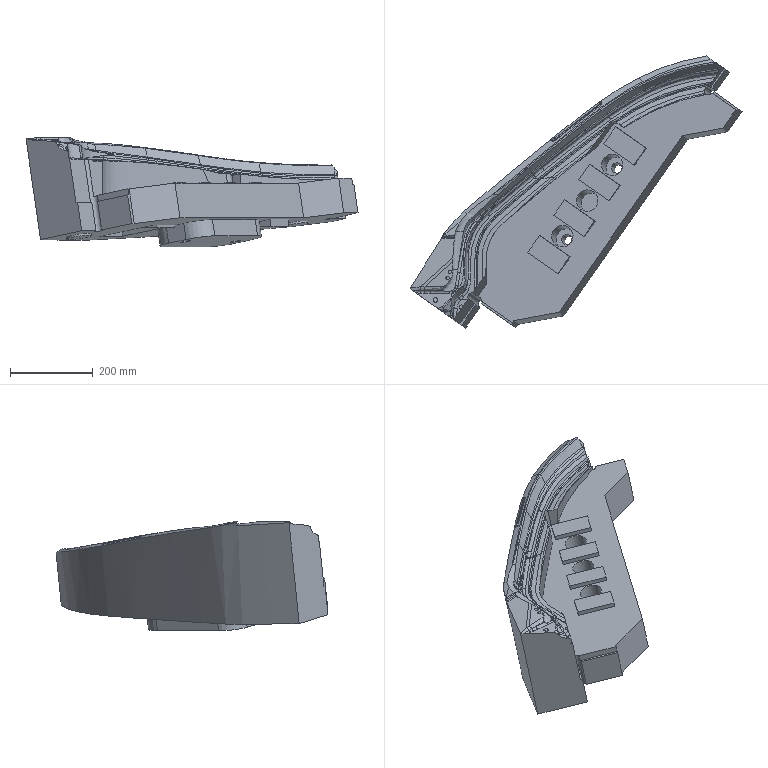Part | NX | features solid 2 | 1 solid | 272 faces | box 800.597 x 655.894 x 264.375 mm | volume 24692181 mm3 | spline 178 | plane 80 | cylinder 14 | commonest cylinder face diameters 100 x4 20 x3 52 x3 25 x2 60 x2